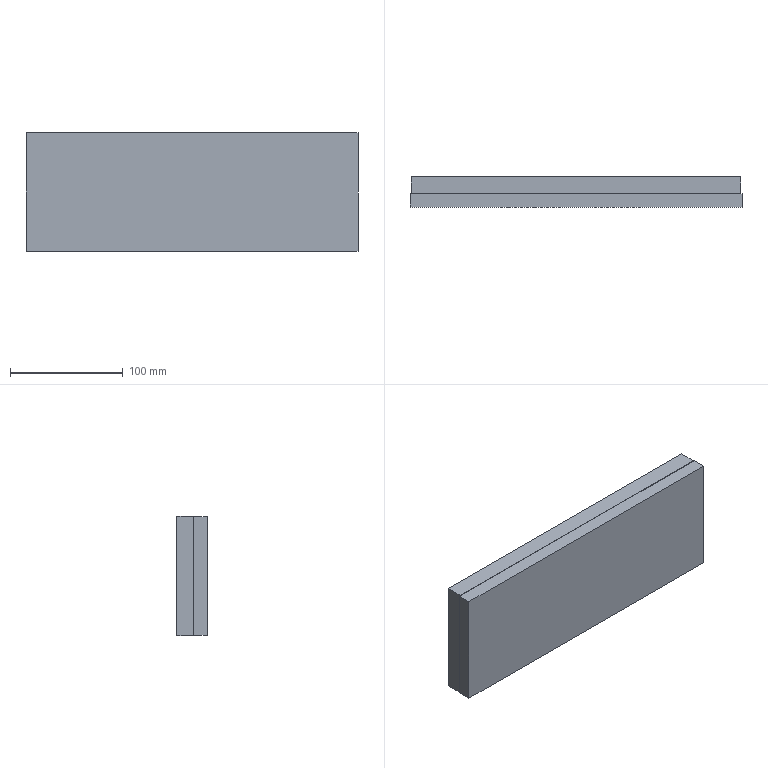NC program | NX | posted with a generic post | part box 295 x 27 x 106 mm
Lines 4615 to 5544 of 7486:
(FLOOR_WALL_6_COPY_COPY , TOOL : D10-L40)
N9012 T04 M6
N9014 G54
N9016 G17 G0 G90 X-0.87 Y66. S6500 M3
N9018 G43 Z16. H4
N9020 Z1.
N9022 G94 G1 Z0. F4000.
N9024 Y54.
N9026 X147.003
N9028 G2 X147.5 Y53.503 R0.5
N9030 G1 Y-53.503
N9032 G2 X147.003 Y-54. R0.5
N9034 G1 X-147.003
N9036 G2 X-147.5 Y-53.503 R0.5
N9038 G1 Y53.503
N9040 G2 X-147.003 Y54. R0.5
N9042 G1 X1.363
N9044 G2 X1.778 Y53.778 R0.5
N9046 G1 X6.482 Y46.722
N9048 G3 X6.897 Y46.5 R0.5
N9050 G1 X139.503
N9052 G2 X140. Y46.003 R0.5
N9054 G1 Y-46.003
N9056 G2 X139.503 Y-46.5 R0.5
N9058 G1 X-109.967
N9060 G2 X-110.311 Y-45.64 R0.5
N9062 G3 X-123.904 Y-45.429 R-9.7
N9064 X-123.408 Y-45.557 R0.5
N9066 G1 X-122.858 Y-45.396
N9068 G3 X-122.655 Y-44.554 R0.5
N9070 G2 X-122.938 Y-32.961 R8.2
N9072 X-122.655 Y-44.554 R-8.2
N9074 G3 X-123.486 Y-44.798 R0.5
N9076 G1 X-123.636 Y-45.42
N9078 G3 X-123.593 Y-45.768 R0.5
N9080 G2 X-124.033 Y-46.5 R0.5
N9082 G1 X-135.475
N9084 X-135.537 Y-46.518
N9086 X-135.567 Y-46.462
N9088 X-135.655 Y-46.373
N9090 X-135.703 Y-46.304
N9092 X-135.786 Y-46.313
N9094 G2 X-138.035 Y-43.173 R2.5
N9096 G1 X-134.95 Y-31.633
N9098 G2 X-131.889 Y-29.863 R2.5
N9100 X-130.119 Y-32.924 R2.5
N9102 G1 X-133.205 Y-44.464
N9104 G2 X-135.48 Y-46.315 R2.5
N9106 G1 X-135.538 Y-46.298
N9108 X-135.565 Y-46.353
N9110 X-135.65 Y-46.439
N9112 X-135.706 Y-46.512
N9114 X-135.797 Y-46.5
N9116 X-139.503
N9118 G2 X-140. Y-46.003 R0.5
N9120 G1 Y46.003
N9122 G2 X-139.503 Y46.5 R0.5
N9124 G1 X1.363
N9126 G2 X1.778 Y46.278 R0.5
N9128 G1 X6.482 Y39.222
N9130 G3 X6.897 Y39. R0.5
N9132 G1 X132.004
N9134 G2 X132.5 Y38.504 R0.5
N9136 G1 Y-38.504
N9138 G2 X132.004 Y-39. R0.5
N9140 G1 X-99.304
N9142 G2 X-99.8 Y-38.507 R0.5
N9144 G3 X-131.578 Y-29.488 R17.2
N9146 G2 X-132.5 Y-29.223 R0.5
N9148 G1 Y38.504
N9150 G2 X-132.004 Y39. R0.5
N9152 G1 X1.363
N9154 G2 X1.778 Y38.778 R0.5
N9156 G1 X6.482 Y31.722
N9158 G3 X6.897 Y31.5 R0.5
N9160 G1 X124.504
N9162 G2 X125. Y31.004 R0.5
N9164 G1 Y-31.004
N9166 G2 X124.504 Y-31.5 R0.5
N9168 G1 X-92.982
N9170 G2 X-93.454 Y-31.155 R0.5
N9172 G3 X-124.355 Y-15.036 R24.7
N9174 G2 X-125. Y-14.561 R0.5
N9176 G1 Y31.004
N9178 G2 X-124.504 Y31.5 R0.5
N9180 G1 X1.363
N9182 G2 X1.778 Y31.278 R0.5
N9184 G1 X6.482 Y24.222
N9186 G3 X6.897 Y24. R0.5
N9188 G1 X117.004
N9190 G2 X117.5 Y23.504 R0.5
N9192 G1 Y-23.504
N9194 G2 X117.004 Y-24. R0.5
N9196 G1 X-88.008
N9198 G2 X-88.445 Y-23.735 R0.5
N9200 G3 X-117.004 Y-6.416 R32.2
N9202 G2 X-117.5 Y-5.92 R0.5
N9204 G1 Y23.504
N9206 G2 X-117.004 Y24. R0.5
N9208 G1 X1.363
N9210 G2 X1.778 Y23.778 R0.5
N9212 G1 X6.482 Y16.722
N9214 G3 X6.897 Y16.5 R0.5
N9216 G1 X93.139
N9218 G2 X93.479 Y16.367 R0.5
N9220 G1 X95.02 Y14.937
N9222 G3 X95.316 Y14.806 R0.5
N9224 G2 X95.95 Y9.963 R2.5
N9226 G1 X89.978 Y7.808
N9228 G2 X86.778 Y9.31 R2.5
N9230 X88.28 Y12.511 R2.5
N9232 G1 X93.262 Y14.309
N9234 G3 X93.477 Y14.46 R0.5
N9236 G1 X95.019 Y16.319
N9238 G2 X95.404 Y16.5 R0.5
N9240 G1 X109.504
N9242 G2 X110. Y16.004 R0.5
N9244 G1 Y6.909
N9246 G2 X109.135 Y6.571 R0.5
N9248 G3 X108.928 Y-6.789 R-9.7
N9250 X109.048 Y-6.291 R0.5
N9252 G1 X108.877 Y-5.744
N9254 G3 X108.032 Y-5.555 R0.5
N9256 G2 X96.445 Y-6.032 R8.2
N9258 X108.032 Y-5.555 R-8.2
N9260 G3 X108.29 Y-6.381 R0.5
N9262 G1 X108.915 Y-6.521
N9264 G3 X109.262 Y-6.473 R0.5
N9266 G2 X110. Y-6.909 R0.5
N9268 G1 Y-16.004
N9270 G2 X109.504 Y-16.5 R0.5
N9272 G1 X95.404
N9274 G2 X95.019 Y-16.319 R0.5
N9276 G1 X93.477 Y-14.46
N9278 G3 X93.262 Y-14.309 R0.5
N9280 G1 X88.28 Y-12.511
N9282 G2 X86.778 Y-9.31 R2.5
N9284 X89.978 Y-7.808 R2.5
N9286 G1 X95.95 Y-9.963
N9288 G2 X95.316 Y-14.806 R2.5
N9290 G3 X95.019 Y-14.937 R0.5
N9292 G1 X93.479 Y-16.367
N9294 G2 X93.139 Y-16.5 R0.5
N9296 G1 X-83.769
N9298 G2 X-84.176 Y-16.285 R0.5
N9300 G3 X-109.598 Y0.388 R39.7
N9302 G2 X-110. Y0.874 R0.5
N9304 G1 Y16.004
N9306 G2 X-109.504 Y16.5 R0.5
N9308 G1 X1.363
N9310 G2 X1.778 Y16.278 R0.5
N9312 G1 X6.482 Y9.222
N9314 G3 X6.897 Y9. R0.5
N9316 G1 X86.479
N9318 G2 X86.915 Y8.264 R0.5
N9320 G3 X86.915 Y-8.264 R17.2
N9322 G2 X86.479 Y-9. R0.5
N9324 G1 X-80.014
N9326 G2 X-80.394 Y-8.819 R0.5
N9328 G3 X-102.162 Y6.191 R47.2
N9330 G2 X-102.5 Y6.66 R0.5
N9332 G1 Y8.505
N9334 G2 X-102.005 Y9. R0.5
N9336 G1 X-89.519
N9338 G2 X-89.136 Y8.822 R0.5
N9340 G1 X-87.551 Y6.941
N9342 G3 X-87.326 Y6.788 R0.5
N9344 G1 X-80.637 Y4.579
N9346 G2 X-79.047 Y1.421 R2.5
N9348 X-82.205 Y-0.168 R2.5
N9350 G1 X-89.917 Y2.379
N9352 G2 X-89.43 Y7.235 R2.5
N9354 G3 X-89.147 Y7.367 R0.5
N9356 G1 X-87.557 Y8.864
N9358 G2 X-87.214 Y9. R0.5
N9360 G1 X1.363
N9362 G2 X1.778 Y8.778 R0.5
N9364 G1 X6.482 Y1.722
N9366 G3 X6.897 Y1.5 R0.5
N9368 G1 X76.825
N9370 G2 X77.32 Y0.985 R0.5
N9372 G3 X77.32 Y-0.985 R24.7
N9374 G2 X76.825 Y-1.5 R0.5
N9376 G1 X-76.606
N9378 G2 X-76.963 Y-1.344 R0.5
N9380 G3 X-78.912 Y0.645 R54.7
N9382 G2 X-78.565 Y1.5 R0.5
N9384 G1 X4.13
N9386 X5.13
N9388 Y13.5
N9390 Z1.
N9392 G0 X-0.87 Y66.
N9394 Z0.7
N9396 G1 Z-0.3
N9398 Y54.
N9400 X147.003
N9402 G2 X147.5 Y53.503 R0.5
N9404 G1 Y-53.503
N9406 G2 X147.003 Y-54. R0.5
N9408 G1 X-147.003
N9410 G2 X-147.5 Y-53.503 R0.5
N9412 G1 Y53.503
N9414 G2 X-147.003 Y54. R0.5
N9416 G1 X4.13
N9418 G2 X4.611 Y53.636 R0.5
N9420 G1 X6.527 Y46.863
N9422 G3 X7.008 Y46.5 R0.5
N9424 G1 X139.503
N9426 G2 X140. Y46.003 R0.5
N9428 G1 Y-46.003
N9430 G2 X139.503 Y-46.5 R0.5
N9432 G1 X-109.967
N9434 G2 X-110.311 Y-45.64 R0.5
N9436 G3 X-123.904 Y-45.429 R-9.7
N9438 X-123.408 Y-45.557 R0.5
N9440 G1 X-122.858 Y-45.396
N9442 G3 X-122.655 Y-44.554 R0.5
N9444 G2 X-122.938 Y-32.961 R8.2
N9446 X-122.655 Y-44.554 R-8.2
N9448 G3 X-123.486 Y-44.798 R0.5
N9450 G1 X-123.636 Y-45.42
N9452 G3 X-123.593 Y-45.768 R0.5
N9454 G2 X-124.033 Y-46.5 R0.5
N9456 G1 X-135.475
N9458 X-135.537 Y-46.518
N9460 X-135.567 Y-46.462
N9462 X-135.655 Y-46.373
N9464 X-135.703 Y-46.304
N9466 X-135.786 Y-46.313
N9468 G2 X-138.035 Y-43.173 R2.5
N9470 G1 X-134.95 Y-31.633
N9472 G2 X-131.889 Y-29.863 R2.5
N9474 X-130.119 Y-32.924 R2.5
N9476 G1 X-133.205 Y-44.464
N9478 G2 X-135.48 Y-46.315 R2.5
N9480 G1 X-135.538 Y-46.298
N9482 X-135.565 Y-46.353
N9484 X-135.65 Y-46.439
N9486 X-135.706 Y-46.512
N9488 X-135.797 Y-46.5
N9490 X-139.503
N9492 G2 X-140. Y-46.003 R0.5
N9494 G1 Y46.003
N9496 G2 X-139.503 Y46.5 R0.5
N9498 G1 X1.363
N9500 G2 X1.778 Y46.278 R0.5
N9502 G1 X6.482 Y39.222
N9504 G3 X6.897 Y39. R0.5
N9506 G1 X132.004
N9508 G2 X132.5 Y38.504 R0.5
N9510 G1 Y-38.504
N9512 G2 X132.004 Y-39. R0.5
N9514 G1 X-99.304
N9516 G2 X-99.8 Y-38.507 R0.5
N9518 G3 X-131.578 Y-29.488 R17.2
N9520 G2 X-132.5 Y-29.223 R0.5
N9522 G1 Y38.504
N9524 G2 X-132.004 Y39. R0.5
N9526 G1 X1.363
N9528 G2 X1.778 Y38.778 R0.5
N9530 G1 X6.482 Y31.722
N9532 G3 X6.897 Y31.5 R0.5
N9534 G1 X124.504
N9536 G2 X125. Y31.004 R0.5
N9538 G1 Y-31.004
N9540 G2 X124.504 Y-31.5 R0.5
N9542 G1 X-92.982
N9544 G2 X-93.454 Y-31.155 R0.5
N9546 G3 X-124.355 Y-15.036 R24.7
N9548 G2 X-125. Y-14.561 R0.5
N9550 G1 Y31.004
N9552 G2 X-124.504 Y31.5 R0.5
N9554 G1 X1.363
N9556 G2 X1.778 Y31.278 R0.5
N9558 G1 X6.482 Y24.222
N9560 G3 X6.897 Y24. R0.5
N9562 G1 X117.004
N9564 G2 X117.5 Y23.504 R0.5
N9566 G1 Y-23.504
N9568 G2 X117.004 Y-24. R0.5
N9570 G1 X-88.008
N9572 G2 X-88.445 Y-23.735 R0.5
N9574 G3 X-117.004 Y-6.416 R32.2
N9576 G2 X-117.5 Y-5.92 R0.5
N9578 G1 Y23.504
N9580 G2 X-117.004 Y24. R0.5
N9582 G1 X1.363
N9584 G2 X1.778 Y23.778 R0.5
N9586 G1 X6.482 Y16.722
N9588 G3 X6.897 Y16.5 R0.5
N9590 G1 X93.139
N9592 G2 X93.479 Y16.367 R0.5
N9594 G1 X95.02 Y14.937
N9596 G3 X95.316 Y14.806 R0.5
N9598 G2 X95.95 Y9.963 R2.5
N9600 G1 X89.978 Y7.808
N9602 G2 X86.778 Y9.31 R2.5
N9604 X88.28 Y12.511 R2.5
N9606 G1 X93.262 Y14.309
N9608 G3 X93.477 Y14.46 R0.5
N9610 G1 X95.019 Y16.319
N9612 G2 X95.404 Y16.5 R0.5
N9614 G1 X109.504
N9616 G2 X110. Y16.004 R0.5
N9618 G1 Y6.909
N9620 G2 X109.135 Y6.571 R0.5
N9622 G3 X108.928 Y-6.789 R-9.7
N9624 X109.048 Y-6.291 R0.5
N9626 G1 X108.877 Y-5.744
N9628 G3 X108.032 Y-5.555 R0.5
N9630 G2 X96.445 Y-6.032 R8.2
N9632 X108.032 Y-5.555 R-8.2
N9634 G3 X108.29 Y-6.381 R0.5
N9636 G1 X108.915 Y-6.521
N9638 G3 X109.262 Y-6.473 R0.5
N9640 G2 X110. Y-6.909 R0.5
N9642 G1 Y-16.004
N9644 G2 X109.504 Y-16.5 R0.5
N9646 G1 X95.404
N9648 G2 X95.019 Y-16.319 R0.5
N9650 G1 X93.477 Y-14.46
N9652 G3 X93.262 Y-14.309 R0.5
N9654 G1 X88.28 Y-12.511
N9656 G2 X86.778 Y-9.31 R2.5
N9658 X89.978 Y-7.808 R2.5
N9660 G1 X95.95 Y-9.963
N9662 G2 X95.316 Y-14.806 R2.5
N9664 G3 X95.019 Y-14.937 R0.5
N9666 G1 X93.479 Y-16.367
N9668 G2 X93.139 Y-16.5 R0.5
N9670 G1 X-83.769
N9672 G2 X-84.176 Y-16.285 R0.5
N9674 G3 X-109.598 Y0.388 R39.7
N9676 G2 X-110. Y0.874 R0.5
N9678 G1 Y16.004
N9680 G2 X-109.504 Y16.5 R0.5
N9682 G1 X1.363
N9684 G2 X1.778 Y16.278 R0.5
N9686 G1 X6.482 Y9.222
N9688 G3 X6.897 Y9. R0.5
N9690 G1 X86.479
N9692 G2 X86.915 Y8.264 R0.5
N9694 G3 X86.915 Y-8.264 R17.2
N9696 G2 X86.479 Y-9. R0.5
N9698 G1 X-80.014
N9700 G2 X-80.394 Y-8.819 R0.5
N9702 G3 X-102.162 Y6.191 R47.2
N9704 G2 X-102.5 Y6.66 R0.5
N9706 G1 Y8.505
N9708 G2 X-102.005 Y9. R0.5
N9710 G1 X-89.519
N9712 G2 X-89.136 Y8.822 R0.5
N9714 G1 X-87.551 Y6.941
N9716 G3 X-87.326 Y6.788 R0.5
N9718 G1 X-80.637 Y4.579
N9720 G2 X-79.047 Y1.421 R2.5
N9722 X-82.205 Y-0.168 R2.5
N9724 G1 X-89.917 Y2.379
N9726 G2 X-89.43 Y7.235 R2.5
N9728 G3 X-89.147 Y7.367 R0.5
N9730 G1 X-87.557 Y8.864
N9732 G2 X-87.214 Y9. R0.5
N9734 G1 X1.363
N9736 G2 X1.778 Y8.778 R0.5
N9738 G1 X6.482 Y1.722
N9740 G3 X6.897 Y1.5 R0.5
N9742 G1 X76.825
N9744 G2 X77.32 Y0.985 R0.5
N9746 G3 X77.32 Y-0.985 R24.7
N9748 G2 X76.825 Y-1.5 R0.5
N9750 G1 X-76.606
N9752 G2 X-76.963 Y-1.344 R0.5
N9754 G3 X-78.912 Y0.645 R54.7
N9756 G2 X-78.565 Y1.5 R0.5
N9758 G1 X4.13
N9760 X5.13
N9762 Y13.5
N9764 Z0.7
N9766 G0 X-0.87 Y66.
N9768 Z0.4
N9770 G1 Z-0.6
N9772 Y54.
N9774 X147.003
N9776 G2 X147.5 Y53.503 R0.5
N9778 G1 Y-53.503
N9780 G2 X147.003 Y-54. R0.5
N9782 G1 X-147.003
N9784 G2 X-147.5 Y-53.503 R0.5
N9786 G1 Y53.503
N9788 G2 X-147.003 Y54. R0.5
N9790 G1 X4.13
N9792 G2 X4.611 Y53.636 R0.5
N9794 G1 X6.527 Y46.863
N9796 G3 X7.008 Y46.5 R0.5
N9798 G1 X139.503
N9800 G2 X140. Y46.003 R0.5
N9802 G1 Y-46.003
N9804 G2 X139.503 Y-46.5 R0.5
N9806 G1 X-109.967
N9808 G2 X-110.311 Y-45.64 R0.5
N9810 G3 X-123.904 Y-45.429 R-9.7
N9812 X-123.408 Y-45.557 R0.5
N9814 G1 X-122.858 Y-45.396
N9816 G3 X-122.655 Y-44.554 R0.5
N9818 G2 X-122.938 Y-32.961 R8.2
N9820 X-122.655 Y-44.554 R-8.2
N9822 G3 X-123.486 Y-44.798 R0.5
N9824 G1 X-123.636 Y-45.42
N9826 G3 X-123.593 Y-45.768 R0.5
N9828 G2 X-124.033 Y-46.5 R0.5
N9830 G1 X-135.475
N9832 X-135.537 Y-46.518
N9834 X-135.567 Y-46.462
N9836 X-135.655 Y-46.373
N9838 X-135.703 Y-46.304
N9840 X-135.786 Y-46.313
N9842 G2 X-138.035 Y-43.173 R2.5
N9844 G1 X-134.95 Y-31.633
N9846 G2 X-131.889 Y-29.863 R2.5
N9848 X-130.119 Y-32.924 R2.5
N9850 G1 X-133.205 Y-44.464
N9852 G2 X-135.48 Y-46.315 R2.5
N9854 G1 X-135.538 Y-46.298
N9856 X-135.565 Y-46.353
N9858 X-135.65 Y-46.439
N9860 X-135.706 Y-46.512
N9862 X-135.797 Y-46.5
N9864 X-139.503
N9866 G2 X-140. Y-46.003 R0.5
N9868 G1 Y46.003
N9870 G2 X-139.503 Y46.5 R0.5
N9872 G1 X1.363
N9874 G2 X1.778 Y46.278 R0.5
N9876 G1 X6.482 Y39.222
N9878 G3 X6.897 Y39. R0.5
N9880 G1 X132.004
N9882 G2 X132.5 Y38.504 R0.5
N9884 G1 Y-38.504
N9886 G2 X132.004 Y-39. R0.5
N9888 G1 X-99.304
N9890 G2 X-99.8 Y-38.507 R0.5
N9892 G3 X-131.578 Y-29.488 R17.2
N9894 G2 X-132.5 Y-29.223 R0.5
N9896 G1 Y38.504
N9898 G2 X-132.004 Y39. R0.5
N9900 G1 X1.363
N9902 G2 X1.778 Y38.778 R0.5
N9904 G1 X6.482 Y31.722
N9906 G3 X6.897 Y31.5 R0.5
N9908 G1 X124.504
N9910 G2 X125. Y31.004 R0.5
N9912 G1 Y-31.004
N9914 G2 X124.504 Y-31.5 R0.5
N9916 G1 X-92.982
N9918 G2 X-93.454 Y-31.155 R0.5
N9920 G3 X-124.355 Y-15.036 R24.7
N9922 G2 X-125. Y-14.561 R0.5
N9924 G1 Y31.004
N9926 G2 X-124.504 Y31.5 R0.5
N9928 G1 X1.363
N9930 G2 X1.778 Y31.278 R0.5
N9932 G1 X6.482 Y24.222
N9934 G3 X6.897 Y24. R0.5
N9936 G1 X117.004
N9938 G2 X117.5 Y23.504 R0.5
N9940 G1 Y-23.504
N9942 G2 X117.004 Y-24. R0.5
N9944 G1 X-88.008
N9946 G2 X-88.445 Y-23.735 R0.5
N9948 G3 X-117.004 Y-6.416 R32.2
N9950 G2 X-117.5 Y-5.92 R0.5
N9952 G1 Y23.504
N9954 G2 X-117.004 Y24. R0.5
N9956 G1 X1.363
N9958 G2 X1.778 Y23.778 R0.5
N9960 G1 X6.482 Y16.722
N9962 G3 X6.897 Y16.5 R0.5
N9964 G1 X93.139
N9966 G2 X93.479 Y16.367 R0.5
N9968 G1 X95.02 Y14.937
N9970 G3 X95.316 Y14.806 R0.5
N9972 G2 X95.95 Y9.963 R2.5
N9974 G1 X89.978 Y7.808
N9976 G2 X86.778 Y9.31 R2.5
N9978 X88.28 Y12.511 R2.5
N9980 G1 X93.262 Y14.309
N9982 G3 X93.477 Y14.46 R0.5
N9984 G1 X95.019 Y16.319
N9986 G2 X95.404 Y16.5 R0.5
N9988 G1 X109.504
N9990 G2 X110. Y16.004 R0.5
N9992 G1 Y6.909
N9994 G2 X109.135 Y6.571 R0.5
N9996 G3 X108.928 Y-6.789 R-9.7
N9998 X109.048 Y-6.291 R0.5
N10000 G1 X108.877 Y-5.744
N10002 G3 X108.032 Y-5.555 R0.5
N10004 G2 X96.445 Y-6.032 R8.2
N10006 X108.032 Y-5.555 R-8.2
N10008 G3 X108.29 Y-6.381 R0.5
N10010 G1 X108.915 Y-6.521
N10012 G3 X109.262 Y-6.473 R0.5
N10014 G2 X110. Y-6.909 R0.5
N10016 G1 Y-16.004
N10018 G2 X109.504 Y-16.5 R0.5
N10020 G1 X95.404
N10022 G2 X95.019 Y-16.319 R0.5
N10024 G1 X93.477 Y-14.46
N10026 G3 X93.262 Y-14.309 R0.5
N10028 G1 X88.28 Y-12.511
N10030 G2 X86.778 Y-9.31 R2.5
N10032 X89.978 Y-7.808 R2.5
N10034 G1 X95.95 Y-9.963
N10036 G2 X95.316 Y-14.806 R2.5
N10038 G3 X95.019 Y-14.937 R0.5
N10040 G1 X93.479 Y-16.367
N10042 G2 X93.139 Y-16.5 R0.5
N10044 G1 X-83.769
N10046 G2 X-84.176 Y-16.285 R0.5
N10048 G3 X-109.598 Y0.388 R39.7
N10050 G2 X-110. Y0.874 R0.5
N10052 G1 Y16.004
N10054 G2 X-109.504 Y16.5 R0.5
N10056 G1 X1.363
N10058 G2 X1.778 Y16.278 R0.5
N10060 G1 X6.482 Y9.222
N10062 G3 X6.897 Y9. R0.5
N10064 G1 X86.479
N10066 G2 X86.915 Y8.264 R0.5
N10068 G3 X86.915 Y-8.264 R17.2
N10070 G2 X86.479 Y-9. R0.5
N10072 G1 X-80.014
N10074 G2 X-80.394 Y-8.819 R0.5
N10076 G3 X-102.162 Y6.191 R47.2
N10078 G2 X-102.5 Y6.66 R0.5
N10080 G1 Y8.505
N10082 G2 X-102.005 Y9. R0.5
N10084 G1 X-89.519
N10086 G2 X-89.136 Y8.822 R0.5
N10088 G1 X-87.551 Y6.941
N10090 G3 X-87.326 Y6.788 R0.5
N10092 G1 X-80.637 Y4.579
N10094 G2 X-79.047 Y1.421 R2.5
N10096 X-82.205 Y-0.168 R2.5
N10098 G1 X-89.917 Y2.379
N10100 G2 X-89.43 Y7.235 R2.5
N10102 G3 X-89.147 Y7.367 R0.5
N10104 G1 X-87.557 Y8.864
N10106 G2 X-87.214 Y9. R0.5
N10108 G1 X1.363
N10110 G2 X1.778 Y8.778 R0.5
N10112 G1 X6.482 Y1.722
N10114 G3 X6.897 Y1.5 R0.5
N10116 G1 X76.825
N10118 G2 X77.32 Y0.985 R0.5
N10120 G3 X77.32 Y-0.985 R24.7
N10122 G2 X76.825 Y-1.5 R0.5
N10124 G1 X-76.606
N10126 G2 X-76.963 Y-1.344 R0.5
N10128 G3 X-78.912 Y0.645 R54.7
N10130 G2 X-78.565 Y1.5 R0.5
N10132 G1 X4.13
N10134 X5.13
N10136 Y13.5
N10138 Z0.4
N10140 G0 X-0.87 Y66.
N10142 Z0.1
N10144 G1 Z-0.9
N10146 Y54.
N10148 X147.003
N10150 G2 X147.5 Y53.503 R0.5
N10152 G1 Y-53.503
N10154 G2 X147.003 Y-54. R0.5
N10156 G1 X-147.003
N10158 G2 X-147.5 Y-53.503 R0.5
N10160 G1 Y53.503
N10162 G2 X-147.003 Y54. R0.5
N10164 G1 X4.13
N10166 G2 X4.611 Y53.636 R0.5
N10168 G1 X6.527 Y46.863
N10170 G3 X7.008 Y46.5 R0.5
N10172 G1 X139.503
N10174 G2 X140. Y46.003 R0.5
N10176 G1 Y-46.003
N10178 G2 X139.503 Y-46.5 R0.5
N10180 G1 X-109.967
N10182 G2 X-110.311 Y-45.64 R0.5
N10184 G3 X-123.904 Y-45.429 R-9.7
N10186 X-123.408 Y-45.557 R0.5
N10188 G1 X-122.858 Y-45.396
N10190 G3 X-122.655 Y-44.554 R0.5
N10192 G2 X-122.938 Y-32.961 R8.2
N10194 X-122.655 Y-44.554 R-8.2
N10196 G3 X-123.486 Y-44.798 R0.5
N10198 G1 X-123.636 Y-45.42
N10200 G3 X-123.593 Y-45.768 R0.5
N10202 G2 X-124.033 Y-46.5 R0.5
N10204 G1 X-135.475
N10206 X-135.537 Y-46.518
N10208 X-135.567 Y-46.462
N10210 X-135.655 Y-46.373
N10212 X-135.703 Y-46.304
N10214 X-135.786 Y-46.313
N10216 G2 X-138.035 Y-43.173 R2.5
N10218 G1 X-134.95 Y-31.633
N10220 G2 X-131.889 Y-29.863 R2.5
N10222 X-130.119 Y-32.924 R2.5
N10224 G1 X-133.205 Y-44.464
N10226 G2 X-135.48 Y-46.315 R2.5
N10228 G1 X-135.538 Y-46.298
N10230 X-135.565 Y-46.353
N10232 X-135.65 Y-46.439
N10234 X-135.706 Y-46.512
N10236 X-135.797 Y-46.5
N10238 X-139.503
N10240 G2 X-140. Y-46.003 R0.5
N10242 G1 Y46.003
N10244 G2 X-139.503 Y46.5 R0.5
N10246 G1 X1.363
N10248 G2 X1.778 Y46.278 R0.5
N10250 G1 X6.482 Y39.222
N10252 G3 X6.897 Y39. R0.5
N10254 G1 X132.004
N10256 G2 X132.5 Y38.504 R0.5
N10258 G1 Y-38.504
N10260 G2 X132.004 Y-39. R0.5
N10262 G1 X-99.304
N10264 G2 X-99.8 Y-38.507 R0.5
N10266 G3 X-131.578 Y-29.488 R17.2
N10268 G2 X-132.5 Y-29.223 R0.5
N10270 G1 Y38.504
N10272 G2 X-132.004 Y39. R0.5
N10274 G1 X1.363
N10276 G2 X1.778 Y38.778 R0.5
N10278 G1 X6.482 Y31.722
N10280 G3 X6.897 Y31.5 R0.5
N10282 G1 X124.504
N10284 G2 X125. Y31.004 R0.5
N10286 G1 Y-31.004
N10288 G2 X124.504 Y-31.5 R0.5
N10290 G1 X-92.982
N10292 G2 X-93.454 Y-31.155 R0.5
N10294 G3 X-124.355 Y-15.036 R24.7
N10296 G2 X-125. Y-14.561 R0.5
N10298 G1 Y31.004
N10300 G2 X-124.504 Y31.5 R0.5
N10302 G1 X1.363
N10304 G2 X1.778 Y31.278 R0.5
N10306 G1 X6.482 Y24.222
N10308 G3 X6.897 Y24. R0.5
N10310 G1 X117.004
N10312 G2 X117.5 Y23.504 R0.5
N10314 G1 Y-23.504
N10316 G2 X117.004 Y-24. R0.5
N10318 G1 X-88.008
N10320 G2 X-88.445 Y-23.735 R0.5
N10322 G3 X-117.004 Y-6.416 R32.2
N10324 G2 X-117.5 Y-5.92 R0.5
N10326 G1 Y23.504
N10328 G2 X-117.004 Y24. R0.5
N10330 G1 X1.363
N10332 G2 X1.778 Y23.778 R0.5
N10334 G1 X6.482 Y16.722
N10336 G3 X6.897 Y16.5 R0.5
N10338 G1 X93.139
N10340 G2 X93.479 Y16.367 R0.5
N10342 G1 X95.02 Y14.937
N10344 G3 X95.316 Y14.806 R0.5
N10346 G2 X95.95 Y9.963 R2.5
N10348 G1 X89.978 Y7.808
N10350 G2 X86.778 Y9.31 R2.5
N10352 X88.28 Y12.511 R2.5
N10354 G1 X93.262 Y14.309
N10356 G3 X93.477 Y14.46 R0.5
N10358 G1 X95.019 Y16.319
N10360 G2 X95.404 Y16.5 R0.5
N10362 G1 X109.504
N10364 G2 X110. Y16.004 R0.5
N10366 G1 Y6.909
N10368 G2 X109.135 Y6.571 R0.5
N10370 G3 X108.928 Y-6.789 R-9.7
N10372 X109.048 Y-6.291 R0.5
N10374 G1 X108.877 Y-5.744
N10376 G3 X108.032 Y-5.555 R0.5
N10378 G2 X96.445 Y-6.032 R8.2
N10380 X108.032 Y-5.555 R-8.2
N10382 G3 X108.29 Y-6.381 R0.5
N10384 G1 X108.915 Y-6.521
N10386 G3 X109.262 Y-6.473 R0.5
N10388 G2 X110. Y-6.909 R0.5
N10390 G1 Y-16.004
N10392 G2 X109.504 Y-16.5 R0.5
N10394 G1 X95.404
N10396 G2 X95.019 Y-16.319 R0.5
N10398 G1 X93.477 Y-14.46
N10400 G3 X93.262 Y-14.309 R0.5
N10402 G1 X88.28 Y-12.511
N10404 G2 X86.778 Y-9.31 R2.5
N10406 X89.978 Y-7.808 R2.5
N10408 G1 X95.95 Y-9.963
N10410 G2 X95.316 Y-14.806 R2.5
N10412 G3 X95.019 Y-14.937 R0.5
N10414 G1 X93.479 Y-16.367
N10416 G2 X93.139 Y-16.5 R0.5
N10418 G1 X-83.769
N10420 G2 X-84.176 Y-16.285 R0.5
N10422 G3 X-109.598 Y0.388 R39.7
N10424 G2 X-110. Y0.874 R0.5
N10426 G1 Y16.004
N10428 G2 X-109.504 Y16.5 R0.5
N10430 G1 X1.363
N10432 G2 X1.778 Y16.278 R0.5
N10434 G1 X6.482 Y9.222
N10436 G3 X6.897 Y9. R0.5
N10438 G1 X86.479
N10440 G2 X86.915 Y8.264 R0.5
N10442 G3 X86.915 Y-8.264 R17.2
N10444 G2 X86.479 Y-9. R0.5
N10446 G1 X-80.014
N10448 G2 X-80.394 Y-8.819 R0.5
N10450 G3 X-102.162 Y6.191 R47.2
N10452 G2 X-102.5 Y6.66 R0.5
N10454 G1 Y8.505
N10456 G2 X-102.005 Y9. R0.5
N10458 G1 X-89.519
N10460 G2 X-89.136 Y8.822 R0.5
N10462 G1 X-87.551 Y6.941
N10464 G3 X-87.326 Y6.788 R0.5
N10466 G1 X-80.637 Y4.579
N10468 G2 X-79.047 Y1.421 R2.5
N10470 X-82.205 Y-0.168 R2.5
N10472 G1 X-89.917 Y2.379
N10474 G2 X-89.43 Y7.235 R2.5
N10476 G3 X-89.147 Y7.367 R0.5
N10478 G1 X-87.557 Y8.864
N10480 G2 X-87.214 Y9. R0.5
N10482 G1 X1.363
N10484 G2 X1.778 Y8.778 R0.5
N10486 G1 X6.482 Y1.722
N10488 G3 X6.897 Y1.5 R0.5
N10490 G1 X76.825
N10492 G2 X77.32 Y0.985 R0.5
N10494 G3 X77.32 Y-0.985 R24.7
N10496 G2 X76.825 Y-1.5 R0.5
N10498 G1 X-76.606
N10500 G2 X-76.963 Y-1.344 R0.5
N10502 G3 X-78.912 Y0.645 R54.7
N10504 G2 X-78.565 Y1.5 R0.5
N10506 G1 X4.13
N10508 X5.13
N10510 Y13.5
N10512 Z0.1
N10514 G0 X-0.87 Y66.
N10516 Z-0.2
N10518 G1 Z-1.2
N10520 Y54.
N10522 X147.003
N10524 G2 X147.5 Y53.503 R0.5
N10526 G1 Y-53.503
N10528 G2 X147.003 Y-54. R0.5
N10530 G1 X-147.003
N10532 G2 X-147.5 Y-53.503 R0.5
N10534 G1 Y53.503
N10536 G2 X-147.003 Y54. R0.5
N10538 G1 X4.13
N10540 G2 X4.611 Y53.636 R0.5
N10542 G1 X6.527 Y46.863
N10544 G3 X7.008 Y46.5 R0.5
N10546 G1 X139.503
N10548 G2 X140. Y46.003 R0.5
N10550 G1 Y-46.003
N10552 G2 X139.503 Y-46.5 R0.5
N10554 G1 X-109.967
N10556 G2 X-110.311 Y-45.64 R0.5
N10558 G3 X-123.904 Y-45.429 R-9.7
N10560 X-123.408 Y-45.557 R0.5
N10562 G1 X-122.858 Y-45.396
N10564 G3 X-122.655 Y-44.554 R0.5
N10566 G2 X-122.938 Y-32.961 R8.2
N10568 X-122.655 Y-44.554 R-8.2
N10570 G3 X-123.486 Y-44.798 R0.5
N10572 G1 X-123.636 Y-45.42
N10574 G3 X-123.593 Y-45.768 R0.5
N10576 G2 X-124.033 Y-46.5 R0.5
N10578 G1 X-135.475
N10580 X-135.537 Y-46.518
N10582 X-135.567 Y-46.462
N10584 X-135.655 Y-46.373
N10586 X-135.703 Y-46.304
N10588 X-135.786 Y-46.313
N10590 G2 X-138.035 Y-43.173 R2.5
N10592 G1 X-134.95 Y-31.633
N10594 G2 X-131.889 Y-29.863 R2.5
N10596 X-130.119 Y-32.924 R2.5
N10598 G1 X-133.205 Y-44.464
N10600 G2 X-135.48 Y-46.315 R2.5
N10602 G1 X-135.538 Y-46.298
N10604 X-135.565 Y-46.353
N10606 X-135.65 Y-46.439
N10608 X-135.706 Y-46.512
N10610 X-135.797 Y-46.5
N10612 X-139.503
N10614 G2 X-140. Y-46.003 R0.5
N10616 G1 Y46.003
N10618 G2 X-139.503 Y46.5 R0.5
N10620 G1 X1.363
N10622 G2 X1.778 Y46.278 R0.5
N10624 G1 X6.482 Y39.222
N10626 G3 X6.897 Y39. R0.5
N10628 G1 X132.004
N10630 G2 X132.5 Y38.504 R0.5
N10632 G1 Y-38.504
N10634 G2 X132.004 Y-39. R0.5
N10636 G1 X-99.304
N10638 G2 X-99.8 Y-38.507 R0.5
N10640 G3 X-131.578 Y-29.488 R17.2
N10642 G2 X-132.5 Y-29.223 R0.5
N10644 G1 Y38.504
N10646 G2 X-132.004 Y39. R0.5
N10648 G1 X1.363
N10650 G2 X1.778 Y38.778 R0.5
N10652 G1 X6.482 Y31.722
N10654 G3 X6.897 Y31.5 R0.5
N10656 G1 X124.504
N10658 G2 X125. Y31.004 R0.5
N10660 G1 Y-31.004
N10662 G2 X124.504 Y-31.5 R0.5
N10664 G1 X-92.982
N10666 G2 X-93.454 Y-31.155 R0.5
N10668 G3 X-124.355 Y-15.036 R24.7
N10670 G2 X-125. Y-14.561 R0.5
N10672 G1 Y31.004
N10674 G2 X-124.504 Y31.5 R0.5
N10676 G1 X1.363
N10678 G2 X1.778 Y31.278 R0.5
N10680 G1 X6.482 Y24.222
N10682 G3 X6.897 Y24. R0.5
N10684 G1 X117.004
N10686 G2 X117.5 Y23.504 R0.5
N10688 G1 Y-23.504
N10690 G2 X117.004 Y-24. R0.5
N10692 G1 X-88.008
N10694 G2 X-88.445 Y-23.735 R0.5
N10696 G3 X-117.004 Y-6.416 R32.2
N10698 G2 X-117.5 Y-5.92 R0.5
N10700 G1 Y23.504
N10702 G2 X-117.004 Y24. R0.5
N10704 G1 X1.363
N10706 G2 X1.778 Y23.778 R0.5
N10708 G1 X6.482 Y16.722
N10710 G3 X6.897 Y16.5 R0.5
N10712 G1 X93.139
N10714 G2 X93.479 Y16.367 R0.5
N10716 G1 X95.02 Y14.937
N10718 G3 X95.316 Y14.806 R0.5
N10720 G2 X95.95 Y9.963 R2.5
N10722 G1 X89.978 Y7.808
N10724 G2 X86.778 Y9.31 R2.5
N10726 X88.28 Y12.511 R2.5
N10728 G1 X93.262 Y14.309
N10730 G3 X93.477 Y14.46 R0.5
N10732 G1 X95.019 Y16.319
N10734 G2 X95.404 Y16.5 R0.5
N10736 G1 X109.504
N10738 G2 X110. Y16.004 R0.5
N10740 G1 Y6.909
N10742 G2 X109.135 Y6.571 R0.5
N10744 G3 X108.928 Y-6.789 R-9.7
N10746 X109.048 Y-6.291 R0.5
N10748 G1 X108.877 Y-5.744
N10750 G3 X108.032 Y-5.555 R0.5
N10752 G2 X96.445 Y-6.032 R8.2
N10754 X108.032 Y-5.555 R-8.2
N10756 G3 X108.29 Y-6.381 R0.5
N10758 G1 X108.915 Y-6.521
N10760 G3 X109.262 Y-6.473 R0.5
N10762 G2 X110. Y-6.909 R0.5
N10764 G1 Y-16.004
N10766 G2 X109.504 Y-16.5 R0.5
N10768 G1 X95.404
N10770 G2 X95.019 Y-16.319 R0.5
N10772 G1 X93.477 Y-14.46
N10774 G3 X93.262 Y-14.309 R0.5
N10776 G1 X88.28 Y-12.511
N10778 G2 X86.778 Y-9.31 R2.5
N10780 X89.978 Y-7.808 R2.5
N10782 G1 X95.95 Y-9.963
N10784 G2 X95.316 Y-14.806 R2.5
N10786 G3 X95.019 Y-14.937 R0.5
N10788 G1 X93.479 Y-16.367
N10790 G2 X93.139 Y-16.5 R0.5
N10792 G1 X-83.769
N10794 G2 X-84.176 Y-16.285 R0.5
N10796 G3 X-109.598 Y0.388 R39.7
N10798 G2 X-110. Y0.874 R0.5
N10800 G1 Y16.004
N10802 G2 X-109.504 Y16.5 R0.5
N10804 G1 X1.363
N10806 G2 X1.778 Y16.278 R0.5
N10808 G1 X6.482 Y9.222
N10810 G3 X6.897 Y9. R0.5
N10812 G1 X86.479
N10814 G2 X86.915 Y8.264 R0.5
N10816 G3 X86.915 Y-8.264 R17.2
N10818 G2 X86.479 Y-9. R0.5
N10820 G1 X-80.014
N10822 G2 X-80.394 Y-8.819 R0.5
N10824 G3 X-102.162 Y6.191 R47.2
N10826 G2 X-102.5 Y6.66 R0.5
N10828 G1 Y8.505
N10830 G2 X-102.005 Y9. R0.5
N10832 G1 X-89.519
N10834 G2 X-89.136 Y8.822 R0.5
N10836 G1 X-87.551 Y6.941
N10838 G3 X-87.326 Y6.788 R0.5
N10840 G1 X-80.637 Y4.579
N10842 G2 X-79.047 Y1.421 R2.5
N10844 X-82.205 Y-0.168 R2.5
N10846 G1 X-89.917 Y2.379
N10848 G2 X-89.43 Y7.235 R2.5
N10850 G3 X-89.147 Y7.367 R0.5
N10852 G1 X-87.557 Y8.864
N10854 G2 X-87.214 Y9. R0.5
N10856 G1 X1.363
N10858 G2 X1.778 Y8.778 R0.5
N10860 G1 X6.482 Y1.722
N10862 G3 X6.897 Y1.5 R0.5
N10864 G1 X76.825